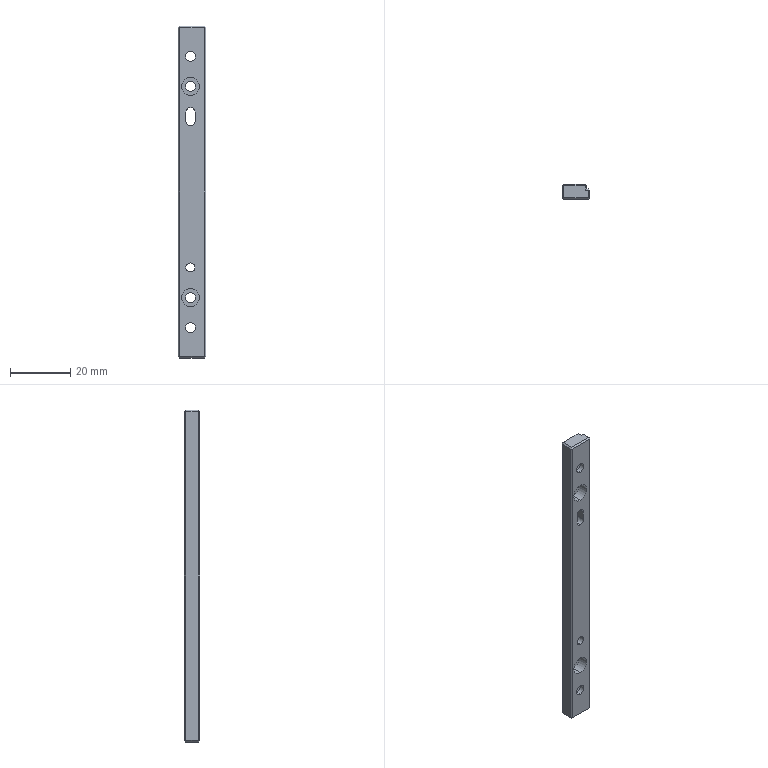Part | SolidWorks | features HoleWzd 3, Chamfer 1, Extrusion 1, ICE 1 | 1 solid | 62 faces | box 9 x 5 x 110 mm | volume 4152 mm3 | plane 41 | cylinder 21 | commonest cylinder face diameters 3.4 x8 6 x8 3 x5